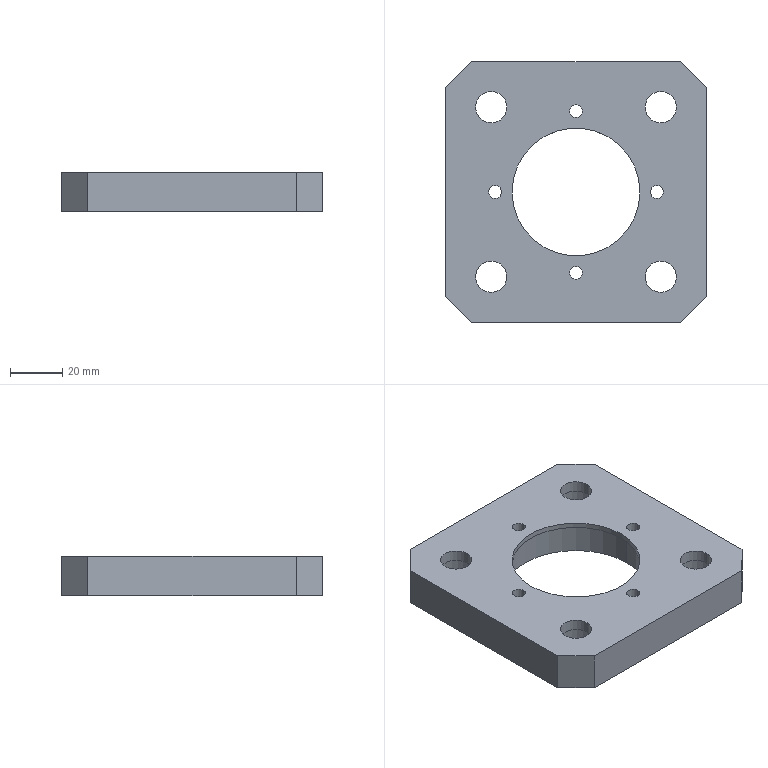Part | SolidWorks | features HoleWzd 2, ICE 2, Chamfer 1, Extrusion 1 | 1 solid | 43 faces | box 100 x 100 x 15 mm | volume 98385 mm3 | cylinder 28 | plane 15 | commonest cylinder face diameters 5 x8 12 x8 18 x8 49 x2 55 x2
STEP:
#1=CARTESIAN_POINT('',(24.5,0.,15.));
#2=VERTEX_POINT('',#1);
#3=CARTESIAN_POINT('',(-24.5,0.,15.));
#4=VERTEX_POINT('',#3);
#5=CARTESIAN_POINT('',(0.,0.,15.));
#6=DIRECTION('',(0.,0.,-1.));
#7=DIRECTION('',(-1.,0.,0.));
#8=AXIS2_PLACEMENT_3D('',#5,#6,#7);
#9=CIRCLE('',#8,24.5);
#10=EDGE_CURVE('',#2,#4,#9,.T.);
#11=ORIENTED_EDGE('',*,*,#10,.F.);
#12=CARTESIAN_POINT('',(24.5,0.,13.));
#13=VERTEX_POINT('',#12);
#14=CARTESIAN_POINT('',(24.5,0.,15.));
#15=DIRECTION('',(0.,0.,-1.));
#16=VECTOR('',#15,1000.);
#17=LINE('',#14,#16);
#18=EDGE_CURVE('',#2,#13,#17,.T.);
#19=ORIENTED_EDGE('',*,*,#18,.T.);
#20=CARTESIAN_POINT('',(-24.5,0.,13.));
#21=VERTEX_POINT('',#20);
#22=CARTESIAN_POINT('',(0.,0.,13.));
#23=DIRECTION('',(0.,0.,-1.));
#24=DIRECTION('',(-1.,0.,0.));
#25=AXIS2_PLACEMENT_3D('',#22,#23,#24);
#26=CIRCLE('',#25,24.5);
#27=EDGE_CURVE('',#13,#21,#26,.T.);
#28=ORIENTED_EDGE('',*,*,#27,.T.);
#29=CARTESIAN_POINT('',(-24.5,0.,15.));
#30=DIRECTION('',(0.,0.,-1.));
#31=VECTOR('',#30,1000.);
#32=LINE('',#29,#31);
#33=EDGE_CURVE('',#4,#21,#32,.T.);
#34=ORIENTED_EDGE('',*,*,#33,.F.);
#35=EDGE_LOOP('',(#11,#19,#28,#34));
#36=FACE_OUTER_BOUND('',#35,.T.);
#37=CARTESIAN_POINT('',(0.,0.,15.));
#38=DIRECTION('',(0.,0.,-1.));
#39=DIRECTION('',(-1.,0.,0.));
#40=AXIS2_PLACEMENT_3D('',#37,#38,#39);
#41=CYLINDRICAL_SURFACE('',#40,24.5);
#42=ADVANCED_FACE('',(#36),#41,.F.);
#43=CARTESIAN_POINT('',(2.5,31.,15.));
#44=VERTEX_POINT('',#43);
#45=CARTESIAN_POINT('',(-2.5,31.,15.));
#46=VERTEX_POINT('',#45);
#47=CARTESIAN_POINT('',(0.,31.,15.));
#48=DIRECTION('',(0.,0.,-1.));
#49=DIRECTION('',(-1.,0.,0.));
#50=AXIS2_PLACEMENT_3D('',#47,#48,#49);
#51=CIRCLE('',#50,2.5);
#52=EDGE_CURVE('',#44,#46,#51,.T.);
#53=ORIENTED_EDGE('',*,*,#52,.F.);
#54=CARTESIAN_POINT('',(2.5,31.,0.));
#55=VERTEX_POINT('',#54);
#56=CARTESIAN_POINT('',(2.5,31.,0.));
#57=DIRECTION('',(0.,0.,-1.));
#58=VECTOR('',#57,1000.);
#59=LINE('',#56,#58);
#60=EDGE_CURVE('',#44,#55,#59,.T.);
#61=ORIENTED_EDGE('',*,*,#60,.T.);
#62=CARTESIAN_POINT('',(-2.5,31.,0.));
#63=VERTEX_POINT('',#62);
#64=CARTESIAN_POINT('',(0.,31.,0.));
#65=DIRECTION('',(0.,0.,-1.));
#66=DIRECTION('',(-1.,0.,0.));
#67=AXIS2_PLACEMENT_3D('',#64,#65,#66);
#68=CIRCLE('',#67,2.5);
#69=EDGE_CURVE('',#55,#63,#68,.T.);
#70=ORIENTED_EDGE('',*,*,#69,.T.);
#71=CARTESIAN_POINT('',(-2.5,31.,0.));
#72=DIRECTION('',(0.,0.,-1.));
#73=VECTOR('',#72,1000.);
#74=LINE('',#71,#73);
#75=EDGE_CURVE('',#46,#63,#74,.T.);
#76=ORIENTED_EDGE('',*,*,#75,.F.);
#77=EDGE_LOOP('',(#53,#61,#70,#76));
#78=FACE_OUTER_BOUND('',#77,.T.);
#79=CARTESIAN_POINT('',(0.,31.,0.));
#80=DIRECTION('',(0.,0.,-1.));
#81=DIRECTION('',(-1.,0.,0.));
#82=AXIS2_PLACEMENT_3D('',#79,#80,#81);
#83=CYLINDRICAL_SURFACE('',#82,2.5);
#84=ADVANCED_FACE('',(#78),#83,.F.);
#85=CARTESIAN_POINT('',(-28.5,0.,15.));
#86=VERTEX_POINT('',#85);
#87=CARTESIAN_POINT('',(-33.5,0.,15.));
#88=VERTEX_POINT('',#87);
#89=CARTESIAN_POINT('',(-31.,0.,15.));
#90=DIRECTION('',(0.,0.,-1.));
#91=DIRECTION('',(-1.,0.,0.));
#92=AXIS2_PLACEMENT_3D('',#89,#90,#91);
#93=CIRCLE('',#92,2.5);
#94=EDGE_CURVE('',#86,#88,#93,.T.);
#95=ORIENTED_EDGE('',*,*,#94,.F.);
#96=CARTESIAN_POINT('',(-28.5,0.,0.));
#97=VERTEX_POINT('',#96);
#98=CARTESIAN_POINT('',(-28.5,0.,0.));
#99=DIRECTION('',(0.,0.,-1.));
#100=VECTOR('',#99,1000.);
#101=LINE('',#98,#100);
#102=EDGE_CURVE('',#86,#97,#101,.T.);
#103=ORIENTED_EDGE('',*,*,#102,.T.);
#104=CARTESIAN_POINT('',(-33.5,0.,0.));
#105=VERTEX_POINT('',#104);
#106=CARTESIAN_POINT('',(-31.,0.,0.));
#107=DIRECTION('',(0.,0.,-1.));
#108=DIRECTION('',(-1.,0.,0.));
#109=AXIS2_PLACEMENT_3D('',#106,#107,#108);
#110=CIRCLE('',#109,2.5);
#111=EDGE_CURVE('',#97,#105,#110,.T.);
#112=ORIENTED_EDGE('',*,*,#111,.T.);
#113=CARTESIAN_POINT('',(-33.5,0.,0.));
#114=DIRECTION('',(0.,0.,-1.));
#115=VECTOR('',#114,1000.);
#116=LINE('',#113,#115);
#117=EDGE_CURVE('',#88,#105,#116,.T.);
#118=ORIENTED_EDGE('',*,*,#117,.F.);
#119=EDGE_LOOP('',(#95,#103,#112,#118));
#120=FACE_OUTER_BOUND('',#119,.T.);
#121=CARTESIAN_POINT('',(-31.,0.,0.));
#122=DIRECTION('',(0.,0.,-1.));
#123=DIRECTION('',(-1.,0.,0.));
#124=AXIS2_PLACEMENT_3D('',#121,#122,#123);
#125=CYLINDRICAL_SURFACE('',#124,2.5);
#126=ADVANCED_FACE('',(#120),#125,.F.);
#127=CARTESIAN_POINT('',(2.5,-31.,15.));
#128=VERTEX_POINT('',#127);
#129=CARTESIAN_POINT('',(-2.5,-31.,15.));
#130=VERTEX_POINT('',#129);
#131=CARTESIAN_POINT('',(0.,-31.,15.));
#132=DIRECTION('',(0.,0.,-1.));
#133=DIRECTION('',(-1.,0.,0.));
#134=AXIS2_PLACEMENT_3D('',#131,#132,#133);
#135=CIRCLE('',#134,2.5);
#136=EDGE_CURVE('',#128,#130,#135,.T.);
#137=ORIENTED_EDGE('',*,*,#136,.F.);
#138=CARTESIAN_POINT('',(2.5,-31.,0.));
#139=VERTEX_POINT('',#138);
#140=CARTESIAN_POINT('',(2.5,-31.,0.));
#141=DIRECTION('',(0.,0.,-1.));
#142=VECTOR('',#141,1000.);
#143=LINE('',#140,#142);
#144=EDGE_CURVE('',#128,#139,#143,.T.);
#145=ORIENTED_EDGE('',*,*,#144,.T.);
#146=CARTESIAN_POINT('',(-2.5,-31.,0.));
#147=VERTEX_POINT('',#146);
#148=CARTESIAN_POINT('',(0.,-31.,0.));
#149=DIRECTION('',(0.,0.,-1.));
#150=DIRECTION('',(-1.,0.,0.));
#151=AXIS2_PLACEMENT_3D('',#148,#149,#150);
#152=CIRCLE('',#151,2.5);
#153=EDGE_CURVE('',#139,#147,#152,.T.);
#154=ORIENTED_EDGE('',*,*,#153,.T.);
#155=CARTESIAN_POINT('',(-2.5,-31.,0.));
#156=DIRECTION('',(0.,0.,-1.));
#157=VECTOR('',#156,1000.);
#158=LINE('',#155,#157);
#159=EDGE_CURVE('',#130,#147,#158,.T.);
#160=ORIENTED_EDGE('',*,*,#159,.F.);
#161=EDGE_LOOP('',(#137,#145,#154,#160));
#162=FACE_OUTER_BOUND('',#161,.T.);
#163=CARTESIAN_POINT('',(0.,-31.,0.));
#164=DIRECTION('',(0.,0.,-1.));
#165=DIRECTION('',(-1.,0.,0.));
#166=AXIS2_PLACEMENT_3D('',#163,#164,#165);
#167=CYLINDRICAL_SURFACE('',#166,2.5);
#168=ADVANCED_FACE('',(#162),#167,.F.);
#169=CARTESIAN_POINT('',(33.5,0.,15.));
#170=VERTEX_POINT('',#169);
#171=CARTESIAN_POINT('',(28.5,0.,15.));
#172=VERTEX_POINT('',#171);
#173=CARTESIAN_POINT('',(31.,0.,15.));
#174=DIRECTION('',(0.,0.,-1.));
#175=DIRECTION('',(-1.,0.,0.));
#176=AXIS2_PLACEMENT_3D('',#173,#174,#175);
#177=CIRCLE('',#176,2.5);
#178=EDGE_CURVE('',#170,#172,#177,.T.);
#179=ORIENTED_EDGE('',*,*,#178,.F.);
#180=CARTESIAN_POINT('',(33.5,0.,0.));
#181=VERTEX_POINT('',#180);
#182=CARTESIAN_POINT('',(33.5,0.,0.));
#183=DIRECTION('',(0.,0.,-1.));
#184=VECTOR('',#183,1000.);
#185=LINE('',#182,#184);
#186=EDGE_CURVE('',#170,#181,#185,.T.);
#187=ORIENTED_EDGE('',*,*,#186,.T.);
#188=CARTESIAN_POINT('',(28.5,0.,0.));
#189=VERTEX_POINT('',#188);
#190=CARTESIAN_POINT('',(31.,0.,0.));
#191=DIRECTION('',(0.,0.,-1.));
#192=DIRECTION('',(-1.,0.,0.));
#193=AXIS2_PLACEMENT_3D('',#190,#191,#192);
#194=CIRCLE('',#193,2.5);
#195=EDGE_CURVE('',#181,#189,#194,.T.);
#196=ORIENTED_EDGE('',*,*,#195,.T.);
#197=CARTESIAN_POINT('',(28.5,0.,0.));
#198=DIRECTION('',(0.,0.,-1.));
#199=VECTOR('',#198,1000.);
#200=LINE('',#197,#199);
#201=EDGE_CURVE('',#172,#189,#200,.T.);
#202=ORIENTED_EDGE('',*,*,#201,.F.);
#203=EDGE_LOOP('',(#179,#187,#196,#202));
#204=FACE_OUTER_BOUND('',#203,.T.);
#205=CARTESIAN_POINT('',(31.,0.,0.));
#206=DIRECTION('',(0.,0.,-1.));
#207=DIRECTION('',(-1.,0.,0.));
#208=AXIS2_PLACEMENT_3D('',#205,#206,#207);
#209=CYLINDRICAL_SURFACE('',#208,2.5);
#210=ADVANCED_FACE('',(#204),#209,.F.);
#211=CARTESIAN_POINT('',(27.5,0.,13.));
#212=VERTEX_POINT('',#211);
#213=CARTESIAN_POINT('',(-27.5,0.,13.));
#214=VERTEX_POINT('',#213);
#215=CARTESIAN_POINT('',(0.,0.,13.));
#216=DIRECTION('',(0.,0.,-1.));
#217=DIRECTION('',(-1.,0.,0.));
#218=AXIS2_PLACEMENT_3D('',#215,#216,#217);
#219=CIRCLE('',#218,27.5);
#220=EDGE_CURVE('',#212,#214,#219,.T.);
#221=ORIENTED_EDGE('',*,*,#220,.F.);
#222=CARTESIAN_POINT('',(27.5,0.,0.));
#223=VERTEX_POINT('',#222);
#224=CARTESIAN_POINT('',(27.5,0.,13.));
#225=DIRECTION('',(0.,0.,-1.));
#226=VECTOR('',#225,1000.);
#227=LINE('',#224,#226);
#228=EDGE_CURVE('',#212,#223,#227,.T.);
#229=ORIENTED_EDGE('',*,*,#228,.T.);
#230=CARTESIAN_POINT('',(-27.5,0.,0.));
#231=VERTEX_POINT('',#230);
#232=CARTESIAN_POINT('',(0.,0.,0.));
#233=DIRECTION('',(0.,0.,-1.));
#234=DIRECTION('',(-1.,0.,0.));
#235=AXIS2_PLACEMENT_3D('',#232,#233,#234);
#236=CIRCLE('',#235,27.5);
#237=EDGE_CURVE('',#223,#231,#236,.T.);
#238=ORIENTED_EDGE('',*,*,#237,.T.);
#239=CARTESIAN_POINT('',(-27.5,0.,13.));
#240=DIRECTION('',(0.,0.,-1.));
#241=VECTOR('',#240,1000.);
#242=LINE('',#239,#241);
#243=EDGE_CURVE('',#214,#231,#242,.T.);
#244=ORIENTED_EDGE('',*,*,#243,.F.);
#245=EDGE_LOOP('',(#221,#229,#238,#244));
#246=FACE_OUTER_BOUND('',#245,.T.);
#247=CARTESIAN_POINT('',(0.,0.,13.));
#248=DIRECTION('',(0.,0.,-1.));
#249=DIRECTION('',(-1.,0.,0.));
#250=AXIS2_PLACEMENT_3D('',#247,#248,#249);
#251=CYLINDRICAL_SURFACE('',#250,27.5);
#252=ADVANCED_FACE('',(#246),#251,.F.);
#253=CARTESIAN_POINT('',(41.5,32.5,10.6));
#254=VERTEX_POINT('',#253);
#255=CARTESIAN_POINT('',(23.5,32.5,10.6));
#256=VERTEX_POINT('',#255);
#257=CARTESIAN_POINT('',(32.5,32.5,10.6));
#258=DIRECTION('',(0.,0.,-1.));
#259=DIRECTION('',(-1.,0.,0.));
#260=AXIS2_PLACEMENT_3D('',#257,#258,#259);
#261=CIRCLE('',#260,9.);
#262=EDGE_CURVE('',#254,#256,#261,.T.);
#263=ORIENTED_EDGE('',*,*,#262,.F.);
#264=CARTESIAN_POINT('',(41.5,32.5,0.));
#265=VERTEX_POINT('',#264);
#266=CARTESIAN_POINT('',(41.5,32.5,0.));
#267=DIRECTION('',(0.,0.,-1.));
#268=VECTOR('',#267,1000.);
#269=LINE('',#266,#268);
#270=EDGE_CURVE('',#254,#265,#269,.T.);
#271=ORIENTED_EDGE('',*,*,#270,.T.);
#272=CARTESIAN_POINT('',(23.5,32.5,0.));
#273=VERTEX_POINT('',#272);
#274=CARTESIAN_POINT('',(32.5,32.5,0.));
#275=DIRECTION('',(0.,0.,-1.));
#276=DIRECTION('',(-1.,0.,0.));
#277=AXIS2_PLACEMENT_3D('',#274,#275,#276);
#278=CIRCLE('',#277,9.);
#279=EDGE_CURVE('',#265,#273,#278,.T.);
#280=ORIENTED_EDGE('',*,*,#279,.T.);
#281=CARTESIAN_POINT('',(23.5,32.5,0.));
#282=DIRECTION('',(0.,0.,-1.));
#283=VECTOR('',#282,1000.);
#284=LINE('',#281,#283);
#285=EDGE_CURVE('',#256,#273,#284,.T.);
#286=ORIENTED_EDGE('',*,*,#285,.F.);
#287=EDGE_LOOP('',(#263,#271,#280,#286));
#288=FACE_OUTER_BOUND('',#287,.T.);
#289=CARTESIAN_POINT('',(32.5,32.5,0.));
#290=DIRECTION('',(0.,0.,-1.));
#291=DIRECTION('',(-1.,0.,0.));
#292=AXIS2_PLACEMENT_3D('',#289,#290,#291);
#293=CYLINDRICAL_SURFACE('',#292,9.);
#294=ADVANCED_FACE('',(#288),#293,.F.);
#295=CARTESIAN_POINT('',(38.5,32.5,15.));
#296=VERTEX_POINT('',#295);
#297=CARTESIAN_POINT('',(26.5,32.5,15.));
#298=VERTEX_POINT('',#297);
#299=CARTESIAN_POINT('',(32.5,32.5,15.));
#300=DIRECTION('',(0.,0.,-1.));
#301=DIRECTION('',(-1.,0.,0.));
#302=AXIS2_PLACEMENT_3D('',#299,#300,#301);
#303=CIRCLE('',#302,6.);
#304=EDGE_CURVE('',#296,#298,#303,.T.);
#305=ORIENTED_EDGE('',*,*,#304,.F.);
#306=CARTESIAN_POINT('',(38.5,32.5,10.6));
#307=VERTEX_POINT('',#306);
#308=CARTESIAN_POINT('',(38.5,32.5,0.));
#309=DIRECTION('',(0.,0.,-1.));
#310=VECTOR('',#309,1000.);
#311=LINE('',#308,#310);
#312=EDGE_CURVE('',#296,#307,#311,.T.);
#313=ORIENTED_EDGE('',*,*,#312,.T.);
#314=CARTESIAN_POINT('',(26.5,32.5,10.6));
#315=VERTEX_POINT('',#314);
#316=CARTESIAN_POINT('',(32.5,32.5,10.6));
#317=DIRECTION('',(0.,0.,-1.));
#318=DIRECTION('',(-1.,0.,0.));
#319=AXIS2_PLACEMENT_3D('',#316,#317,#318);
#320=CIRCLE('',#319,6.);
#321=EDGE_CURVE('',#307,#315,#320,.T.);
#322=ORIENTED_EDGE('',*,*,#321,.T.);
#323=CARTESIAN_POINT('',(26.5,32.5,0.));
#324=DIRECTION('',(0.,0.,-1.));
#325=VECTOR('',#324,1000.);
#326=LINE('',#323,#325);
#327=EDGE_CURVE('',#298,#315,#326,.T.);
#328=ORIENTED_EDGE('',*,*,#327,.F.);
#329=EDGE_LOOP('',(#305,#313,#322,#328));
#330=FACE_OUTER_BOUND('',#329,.T.);
#331=CARTESIAN_POINT('',(32.5,32.5,0.));
#332=DIRECTION('',(0.,0.,-1.));
#333=DIRECTION('',(-1.,0.,0.));
#334=AXIS2_PLACEMENT_3D('',#331,#332,#333);
#335=CYLINDRICAL_SURFACE('',#334,6.);
#336=ADVANCED_FACE('',(#330),#335,.F.);
#337=CARTESIAN_POINT('',(-23.5,32.5,10.6));
#338=VERTEX_POINT('',#337);
#339=CARTESIAN_POINT('',(-41.5,32.5,10.6));
#340=VERTEX_POINT('',#339);
#341=CARTESIAN_POINT('',(-32.5,32.5,10.6));
#342=DIRECTION('',(0.,0.,-1.));
#343=DIRECTION('',(-1.,0.,0.));
#344=AXIS2_PLACEMENT_3D('',#341,#342,#343);
#345=CIRCLE('',#344,9.);
#346=EDGE_CURVE('',#338,#340,#345,.T.);
#347=ORIENTED_EDGE('',*,*,#346,.F.);
#348=CARTESIAN_POINT('',(-23.5,32.5,0.));
#349=VERTEX_POINT('',#348);
#350=CARTESIAN_POINT('',(-23.5,32.5,0.));
#351=DIRECTION('',(0.,0.,-1.));
#352=VECTOR('',#351,1000.);
#353=LINE('',#350,#352);
#354=EDGE_CURVE('',#338,#349,#353,.T.);
#355=ORIENTED_EDGE('',*,*,#354,.T.);
#356=CARTESIAN_POINT('',(-41.5,32.5,0.));
#357=VERTEX_POINT('',#356);
#358=CARTESIAN_POINT('',(-32.5,32.5,0.));
#359=DIRECTION('',(0.,0.,-1.));
#360=DIRECTION('',(-1.,0.,0.));
#361=AXIS2_PLACEMENT_3D('',#358,#359,#360);
#362=CIRCLE('',#361,9.);
#363=EDGE_CURVE('',#349,#357,#362,.T.);
#364=ORIENTED_EDGE('',*,*,#363,.T.);
#365=CARTESIAN_POINT('',(-41.5,32.5,0.));
#366=DIRECTION('',(0.,0.,-1.));
#367=VECTOR('',#366,1000.);
#368=LINE('',#365,#367);
#369=EDGE_CURVE('',#340,#357,#368,.T.);
#370=ORIENTED_EDGE('',*,*,#369,.F.);
#371=EDGE_LOOP('',(#347,#355,#364,#370));
#372=FACE_OUTER_BOUND('',#371,.T.);
#373=CARTESIAN_POINT('',(-32.5,32.5,0.));
#374=DIRECTION('',(0.,0.,-1.));
#375=DIRECTION('',(-1.,0.,0.));
#376=AXIS2_PLACEMENT_3D('',#373,#374,#375);
#377=CYLINDRICAL_SURFACE('',#376,9.);
#378=ADVANCED_FACE('',(#372),#377,.F.);
#379=CARTESIAN_POINT('',(-26.5,32.5,15.));
#380=VERTEX_POINT('',#379);
#381=CARTESIAN_POINT('',(-38.5,32.5,15.));
#382=VERTEX_POINT('',#381);
#383=CARTESIAN_POINT('',(-32.5,32.5,15.));
#384=DIRECTION('',(0.,0.,-1.));
#385=DIRECTION('',(-1.,0.,0.));
#386=AXIS2_PLACEMENT_3D('',#383,#384,#385);
#387=CIRCLE('',#386,6.);
#388=EDGE_CURVE('',#380,#382,#387,.T.);
#389=ORIENTED_EDGE('',*,*,#388,.F.);
#390=CARTESIAN_POINT('',(-26.5,32.5,10.6));
#391=VERTEX_POINT('',#390);
#392=CARTESIAN_POINT('',(-26.5,32.5,0.));
#393=DIRECTION('',(0.,0.,-1.));
#394=VECTOR('',#393,1000.);
#395=LINE('',#392,#394);
#396=EDGE_CURVE('',#380,#391,#395,.T.);
#397=ORIENTED_EDGE('',*,*,#396,.T.);
#398=CARTESIAN_POINT('',(-38.5,32.5,10.6));
#399=VERTEX_POINT('',#398);
#400=CARTESIAN_POINT('',(-32.5,32.5,10.6));
#401=DIRECTION('',(0.,0.,-1.));
#402=DIRECTION('',(-1.,0.,0.));
#403=AXIS2_PLACEMENT_3D('',#400,#401,#402);
#404=CIRCLE('',#403,6.);
#405=EDGE_CURVE('',#391,#399,#404,.T.);
#406=ORIENTED_EDGE('',*,*,#405,.T.);
#407=CARTESIAN_POINT('',(-38.5,32.5,0.));
#408=DIRECTION('',(0.,0.,-1.));
#409=VECTOR('',#408,1000.);
#410=LINE('',#407,#409);
#411=EDGE_CURVE('',#382,#399,#410,.T.);
#412=ORIENTED_EDGE('',*,*,#411,.F.);
#413=EDGE_LOOP('',(#389,#397,#406,#412));
#414=FACE_OUTER_BOUND('',#413,.T.);
#415=CARTESIAN_POINT('',(-32.5,32.5,0.));
#416=DIRECTION('',(0.,0.,-1.));
#417=DIRECTION('',(-1.,0.,0.));
#418=AXIS2_PLACEMENT_3D('',#415,#416,#417);
#419=CYLINDRICAL_SURFACE('',#418,6.);
#420=ADVANCED_FACE('',(#414),#419,.F.);
#421=CARTESIAN_POINT('',(-23.5,-32.5,10.6));
#422=VERTEX_POINT('',#421);
#423=CARTESIAN_POINT('',(-41.5,-32.5,10.6));
#424=VERTEX_POINT('',#423);
#425=CARTESIAN_POINT('',(-32.5,-32.5,10.6));
#426=DIRECTION('',(0.,0.,-1.));
#427=DIRECTION('',(-1.,0.,0.));
#428=AXIS2_PLACEMENT_3D('',#425,#426,#427);
#429=CIRCLE('',#428,9.);
#430=EDGE_CURVE('',#422,#424,#429,.T.);
#431=ORIENTED_EDGE('',*,*,#430,.F.);
#432=CARTESIAN_POINT('',(-23.5,-32.5,0.));
#433=VERTEX_POINT('',#432);
#434=CARTESIAN_POINT('',(-23.5,-32.5,0.));
#435=DIRECTION('',(0.,0.,-1.));
#436=VECTOR('',#435,1000.);
#437=LINE('',#434,#436);
#438=EDGE_CURVE('',#422,#433,#437,.T.);
#439=ORIENTED_EDGE('',*,*,#438,.T.);
#440=CARTESIAN_POINT('',(-41.5,-32.5,0.));
#441=VERTEX_POINT('',#440);
#442=CARTESIAN_POINT('',(-32.5,-32.5,0.));
#443=DIRECTION('',(0.,0.,-1.));
#444=DIRECTION('',(-1.,0.,0.));
#445=AXIS2_PLACEMENT_3D('',#442,#443,#444);
#446=CIRCLE('',#445,9.);
#447=EDGE_CURVE('',#433,#441,#446,.T.);
#448=ORIENTED_EDGE('',*,*,#447,.T.);
#449=CARTESIAN_POINT('',(-41.5,-32.5,0.));
#450=DIRECTION('',(0.,0.,-1.));
#451=VECTOR('',#450,1000.);
#452=LINE('',#449,#451);
#453=EDGE_CURVE('',#424,#441,#452,.T.);
#454=ORIENTED_EDGE('',*,*,#453,.F.);
#455=EDGE_LOOP('',(#431,#439,#448,#454));
#456=FACE_OUTER_BOUND('',#455,.T.);
#457=CARTESIAN_POINT('',(-32.5,-32.5,0.));
#458=DIRECTION('',(0.,0.,-1.));
#459=DIRECTION('',(-1.,0.,0.));
#460=AXIS2_PLACEMENT_3D('',#457,#458,#459);
#461=CYLINDRICAL_SURFACE('',#460,9.);
#462=ADVANCED_FACE('',(#456),#461,.F.);
#463=CARTESIAN_POINT('',(-26.5,-32.5,15.));
#464=VERTEX_POINT('',#463);
#465=CARTESIAN_POINT('',(-38.5,-32.5,15.));
#466=VERTEX_POINT('',#465);
#467=CARTESIAN_POINT('',(-32.5,-32.5,15.));
#468=DIRECTION('',(0.,0.,-1.));
#469=DIRECTION('',(-1.,0.,0.));
#470=AXIS2_PLACEMENT_3D('',#467,#468,#469);
#471=CIRCLE('',#470,6.);
#472=EDGE_CURVE('',#464,#466,#471,.T.);
#473=ORIENTED_EDGE('',*,*,#472,.F.);
#474=CARTESIAN_POINT('',(-26.5,-32.5,10.6));
#475=VERTEX_POINT('',#474);
#476=CARTESIAN_POINT('',(-26.5,-32.5,0.));
#477=DIRECTION('',(0.,0.,-1.));
#478=VECTOR('',#477,1000.);
#479=LINE('',#476,#478);
#480=EDGE_CURVE('',#464,#475,#479,.T.);
#481=ORIENTED_EDGE('',*,*,#480,.T.);
#482=CARTESIAN_POINT('',(-38.5,-32.5,10.6));
#483=VERTEX_POINT('',#482);
#484=CARTESIAN_POINT('',(-32.5,-32.5,10.6));
#485=DIRECTION('',(0.,0.,-1.));
#486=DIRECTION('',(-1.,0.,0.));
#487=AXIS2_PLACEMENT_3D('',#484,#485,#486);
#488=CIRCLE('',#487,6.);
#489=EDGE_CURVE('',#475,#483,#488,.T.);
#490=ORIENTED_EDGE('',*,*,#489,.T.);
#491=CARTESIAN_POINT('',(-38.5,-32.5,0.));
#492=DIRECTION('',(0.,0.,-1.));
#493=VECTOR('',#492,1000.);
#494=LINE('',#491,#493);
#495=EDGE_CURVE('',#466,#483,#494,.T.);
#496=ORIENTED_EDGE('',*,*,#495,.F.);
#497=EDGE_LOOP('',(#473,#481,#490,#496));
#498=FACE_OUTER_BOUND('',#497,.T.);
#499=CARTESIAN_POINT('',(-32.5,-32.5,0.));
#500=DIRECTION('',(0.,0.,-1.));
#501=DIRECTION('',(-1.,0.,0.));
#502=AXIS2_PLACEMENT_3D('',#499,#500,#501);
#503=CYLINDRICAL_SURFACE('',#502,6.);
#504=ADVANCED_FACE('',(#498),#503,.F.);
#505=CARTESIAN_POINT('',(41.5,-32.5,10.6));
#506=VERTEX_POINT('',#505);
#507=CARTESIAN_POINT('',(23.5,-32.5,10.6));
#508=VERTEX_POINT('',#507);
#509=CARTESIAN_POINT('',(32.5,-32.5,10.6));
#510=DIRECTION('',(0.,0.,-1.));
#511=DIRECTION('',(-1.,0.,0.));
#512=AXIS2_PLACEMENT_3D('',#509,#510,#511);
#513=CIRCLE('',#512,9.);
#514=EDGE_CURVE('',#506,#508,#513,.T.);
#515=ORIENTED_EDGE('',*,*,#514,.F.);
#516=CARTESIAN_POINT('',(41.5,-32.5,0.));
#517=VERTEX_POINT('',#516);
#518=CARTESIAN_POINT('',(41.5,-32.5,0.));
#519=DIRECTION('',(0.,0.,-1.));
#520=VECTOR('',#519,1000.);
#521=LINE('',#518,#520);
#522=EDGE_CURVE('',#506,#517,#521,.T.);
#523=ORIENTED_EDGE('',*,*,#522,.T.);
#524=CARTESIAN_POINT('',(23.5,-32.5,0.));
#525=VERTEX_POINT('',#524);
#526=CARTESIAN_POINT('',(32.5,-32.5,0.));
#527=DIRECTION('',(0.,0.,-1.));
#528=DIRECTION('',(-1.,0.,0.));
#529=AXIS2_PLACEMENT_3D('',#526,#527,#528);
#530=CIRCLE('',#529,9.);
#531=EDGE_CURVE('',#517,#525,#530,.T.);
#532=ORIENTED_EDGE('',*,*,#531,.T.);
#533=CARTESIAN_POINT('',(23.5,-32.5,0.));
#534=DIRECTION('',(0.,0.,-1.));
#535=VECTOR('',#534,1000.);
#536=LINE('',#533,#535);
#537=EDGE_CURVE('',#508,#525,#536,.T.);
#538=ORIENTED_EDGE('',*,*,#537,.F.);
#539=EDGE_LOOP('',(#515,#523,#532,#538));
#540=FACE_OUTER_BOUND('',#539,.T.);
#541=CARTESIAN_POINT('',(32.5,-32.5,0.));
#542=DIRECTION('',(0.,0.,-1.));
#543=DIRECTION('',(-1.,0.,0.));
#544=AXIS2_PLACEMENT_3D('',#541,#542,#543);
#545=CYLINDRICAL_SURFACE('',#544,9.);
#546=ADVANCED_FACE('',(#540),#545,.F.);
#547=CARTESIAN_POINT('',(38.5,-32.5,15.));
#548=VERTEX_POINT('',#547);
#549=CARTESIAN_POINT('',(26.5,-32.5,15.));
#550=VERTEX_POINT('',#549);
#551=CARTESIAN_POINT('',(32.5,-32.5,15.));
#552=DIRECTION('',(0.,0.,-1.));
#553=DIRECTION('',(-1.,0.,0.));
#554=AXIS2_PLACEMENT_3D('',#551,#552,#553);
#555=CIRCLE('',#554,6.);
#556=EDGE_CURVE('',#548,#550,#555,.T.);
#557=ORIENTED_EDGE('',*,*,#556,.F.);
#558=CARTESIAN_POINT('',(38.5,-32.5,10.6));
#559=VERTEX_POINT('',#558);
#560=CARTESIAN_POINT('',(38.5,-32.5,0.));
#561=DIRECTION('',(0.,0.,-1.));
#562=VECTOR('',#561,1000.);
#563=LINE('',#560,#562);
#564=EDGE_CURVE('',#548,#559,#563,.T.);
#565=ORIENTED_EDGE('',*,*,#564,.T.);
#566=CARTESIAN_POINT('',(26.5,-32.5,10.6));
#567=VERTEX_POINT('',#566);
#568=CARTESIAN_POINT('',(32.5,-32.5,10.6));
#569=DIRECTION('',(0.,0.,-1.));
#570=DIRECTION('',(-1.,0.,0.));
#571=AXIS2_PLACEMENT_3D('',#568,#569,#570);
#572=CIRCLE('',#571,6.);
#573=EDGE_CURVE('',#559,#567,#572,.T.);
#574=ORIENTED_EDGE('',*,*,#573,.T.);
#575=CARTESIAN_POINT('',(26.5,-32.5,0.));
#576=DIRECTION('',(0.,0.,-1.));
#577=VECTOR('',#576,1000.);
#578=LINE('',#575,#577);
#579=EDGE_CURVE('',#550,#567,#578,.T.);
#580=ORIENTED_EDGE('',*,*,#579,.F.);
#581=EDGE_LOOP('',(#557,#565,#574,#580));
#582=FACE_OUTER_BOUND('',#581,.T.);
#583=CARTESIAN_POINT('',(32.5,-32.5,0.));
#584=DIRECTION('',(0.,0.,-1.));
#585=DIRECTION('',(-1.,0.,0.));
#586=AXIS2_PLACEMENT_3D('',#583,#584,#585);
#587=CYLINDRICAL_SURFACE('',#586,6.);
#588=ADVANCED_FACE('',(#582),#587,.F.);
#589=CARTESIAN_POINT('',(50.,-40.,15.));
#590=VERTEX_POINT('',#589);
#591=CARTESIAN_POINT('',(50.,40.,15.));
#592=VERTEX_POINT('',#591);
#593=CARTESIAN_POINT('',(50.,-50.,15.));
#594=DIRECTION('',(0.,1.,0.));
#595=VECTOR('',#594,1000.);
#596=LINE('',#593,#595);
#597=EDGE_CURVE('',#590,#592,#596,.T.);
#598=ORIENTED_EDGE('',*,*,#597,.F.);
#599=CARTESIAN_POINT('',(50.,-40.,0.));
#600=VERTEX_POINT('',#599);
#601=CARTESIAN_POINT('',(50.,-40.,15.));
#602=DIRECTION('',(0.,0.,-1.));
#603=VECTOR('',#602,1000.);
#604=LINE('',#601,#603);
#605=EDGE_CURVE('',#590,#600,#604,.T.);
#606=ORIENTED_EDGE('',*,*,#605,.T.);
#607=CARTESIAN_POINT('',(50.,40.,0.));
#608=VERTEX_POINT('',#607);
#609=CARTESIAN_POINT('',(50.,-50.,0.));
#610=DIRECTION('',(0.,1.,0.));
#611=VECTOR('',#610,1000.);
#612=LINE('',#609,#611);
#613=EDGE_CURVE('',#600,#608,#612,.T.);
#614=ORIENTED_EDGE('',*,*,#613,.T.);
#615=CARTESIAN_POINT('',(50.,40.,15.));
#616=DIRECTION('',(0.,0.,1.));
#617=VECTOR('',#616,1000.);
#618=LINE('',#615,#617);
#619=EDGE_CURVE('',#608,#592,#618,.T.);
#620=ORIENTED_EDGE('',*,*,#619,.T.);
#621=EDGE_LOOP('',(#598,#606,#614,#620));
#622=FACE_OUTER_BOUND('',#621,.T.);
#623=CARTESIAN_POINT('',(50.,-50.,15.));
#624=DIRECTION('',(-1.,0.,0.));
#625=DIRECTION('',(0.,0.,1.));
#626=AXIS2_PLACEMENT_3D('',#623,#624,#625);
#627=PLANE('',#626);
#628=ADVANCED_FACE('',(#622),#627,.F.);
#629=CARTESIAN_POINT('',(40.,50.,0.));
#630=VERTEX_POINT('',#629);
#631=CARTESIAN_POINT('',(-40.,50.,0.));
#632=VERTEX_POINT('',#631);
#633=CARTESIAN_POINT('',(-50.,50.,0.));
#634=DIRECTION('',(-1.,0.,0.));
#635=VECTOR('',#634,1000.);
#636=LINE('',#633,#635);
#637=EDGE_CURVE('',#630,#632,#636,.T.);
#638=ORIENTED_EDGE('',*,*,#637,.T.);
#639=CARTESIAN_POINT('',(-40.,50.,15.));
#640=VERTEX_POINT('',#639);
#641=CARTESIAN_POINT('',(-40.,50.,15.));
#642=DIRECTION('',(0.,0.,1.));
#643=VECTOR('',#642,1000.);
#644=LINE('',#641,#643);
#645=EDGE_CURVE('',#632,#640,#644,.T.);
#646=ORIENTED_EDGE('',*,*,#645,.T.);
#647=CARTESIAN_POINT('',(40.,50.,15.));
#648=VERTEX_POINT('',#647);
#649=CARTESIAN_POINT('',(-50.,50.,15.));
#650=DIRECTION('',(-1.,0.,0.));
#651=VECTOR('',#650,1000.);
#652=LINE('',#649,#651);
#653=EDGE_CURVE('',#648,#640,#652,.T.);
#654=ORIENTED_EDGE('',*,*,#653,.F.);
#655=CARTESIAN_POINT('',(40.,50.,15.));
#656=DIRECTION('',(0.,0.,-1.));
#657=VECTOR('',#656,1000.);
#658=LINE('',#655,#657);
#659=EDGE_CURVE('',#648,#630,#658,.T.);
#660=ORIENTED_EDGE('',*,*,#659,.T.);
#661=EDGE_LOOP('',(#638,#646,#654,#660));
#662=FACE_OUTER_BOUND('',#661,.T.);
#663=CARTESIAN_POINT('',(-50.,50.,15.));
#664=DIRECTION('',(0.,-1.,0.));
#665=DIRECTION('',(0.,0.,-1.));
#666=AXIS2_PLACEMENT_3D('',#663,#664,#665);
#667=PLANE('',#666);
#668=ADVANCED_FACE('',(#662),#667,.F.);
#669=CARTESIAN_POINT('',(-50.,40.,0.));
#670=VERTEX_POINT('',#669);
#671=CARTESIAN_POINT('',(-50.,-40.,0.));
#672=VERTEX_POINT('',#671);
#673=CARTESIAN_POINT('',(-50.,-50.,0.));
#674=DIRECTION('',(0.,-1.,0.));
#675=VECTOR('',#674,1000.);
#676=LINE('',#673,#675);
#677=EDGE_CURVE('',#670,#672,#676,.T.);
#678=ORIENTED_EDGE('',*,*,#677,.T.);
#679=CARTESIAN_POINT('',(-50.,-40.,15.));
#680=VERTEX_POINT('',#679);
#681=CARTESIAN_POINT('',(-50.,-40.,15.));
#682=DIRECTION('',(0.,0.,1.));
#683=VECTOR('',#682,1000.);
#684=LINE('',#681,#683);
#685=EDGE_CURVE('',#672,#680,#684,.T.);
#686=ORIENTED_EDGE('',*,*,#685,.T.);
#687=CARTESIAN_POINT('',(-50.,40.,15.));
#688=VERTEX_POINT('',#687);
#689=CARTESIAN_POINT('',(-50.,-50.,15.));
#690=DIRECTION('',(0.,-1.,0.));
#691=VECTOR('',#690,1000.);
#692=LINE('',#689,#691);
#693=EDGE_CURVE('',#688,#680,#692,.T.);
#694=ORIENTED_EDGE('',*,*,#693,.F.);
#695=CARTESIAN_POINT('',(-50.,40.,15.));
#696=DIRECTION('',(0.,0.,-1.));
#697=VECTOR('',#696,1000.);
#698=LINE('',#695,#697);
#699=EDGE_CURVE('',#688,#670,#698,.T.);
#700=ORIENTED_EDGE('',*,*,#699,.T.);
#701=EDGE_LOOP('',(#678,#686,#694,#700));
#702=FACE_OUTER_BOUND('',#701,.T.);
#703=CARTESIAN_POINT('',(-50.,-50.,15.));
#704=DIRECTION('',(1.,0.,0.));
#705=DIRECTION('',(0.,0.,-1.));
#706=AXIS2_PLACEMENT_3D('',#703,#704,#705);
#707=PLANE('',#706);
#708=ADVANCED_FACE('',(#702),#707,.F.);
#709=CARTESIAN_POINT('',(-40.,-50.,0.));
#710=VERTEX_POINT('',#709);
#711=CARTESIAN_POINT('',(40.,-50.,0.));
#712=VERTEX_POINT('',#711);
#713=CARTESIAN_POINT('',(-50.,-50.,0.));
#714=DIRECTION('',(1.,0.,0.));
#715=VECTOR('',#714,1000.);
#716=LINE('',#713,#715);
#717=EDGE_CURVE('',#710,#712,#716,.T.);
#718=ORIENTED_EDGE('',*,*,#717,.T.);
#719=CARTESIAN_POINT('',(40.,-50.,15.));
#720=VERTEX_POINT('',#719);
#721=CARTESIAN_POINT('',(40.,-50.,15.));
#722=DIRECTION('',(0.,0.,1.));
#723=VECTOR('',#722,1000.);
#724=LINE('',#721,#723);
#725=EDGE_CURVE('',#712,#720,#724,.T.);
#726=ORIENTED_EDGE('',*,*,#725,.T.);
#727=CARTESIAN_POINT('',(-40.,-50.,15.));
#728=VERTEX_POINT('',#727);
#729=CARTESIAN_POINT('',(-50.,-50.,15.));
#730=DIRECTION('',(1.,0.,0.));
#731=VECTOR('',#730,1000.);
#732=LINE('',#729,#731);
#733=EDGE_CURVE('',#728,#720,#732,.T.);
#734=ORIENTED_EDGE('',*,*,#733,.F.);
#735=CARTESIAN_POINT('',(-40.,-50.,15.));
#736=DIRECTION('',(0.,0.,-1.));
#737=VECTOR('',#736,1000.);
#738=LINE('',#735,#737);
#739=EDGE_CURVE('',#728,#710,#738,.T.);
#740=ORIENTED_EDGE('',*,*,#739,.T.);
#741=EDGE_LOOP('',(#718,#726,#734,#740));
#742=FACE_OUTER_BOUND('',#741,.T.);
#743=CARTESIAN_POINT('',(-50.,-50.,15.));
#744=DIRECTION('',(0.,1.,0.));
#745=DIRECTION('',(0.,0.,1.));
#746=AXIS2_PLACEMENT_3D('',#743,#744,#745);
#747=PLANE('',#746);
#748=ADVANCED_FACE('',(#742),#747,.F.);
#749=CARTESIAN_POINT('',(0.,0.,15.));
#750=DIRECTION('',(0.,0.,-1.));
#751=DIRECTION('',(-1.,0.,0.));
#752=AXIS2_PLACEMENT_3D('',#749,#750,#751);
#753=CIRCLE('',#752,24.5);
#754=EDGE_CURVE('',#4,#2,#753,.T.);
#755=ORIENTED_EDGE('',*,*,#754,.T.);
#756=ORIENTED_EDGE('',*,*,#10,.T.);
#757=EDGE_LOOP('',(#755,#756));
#758=FACE_BOUND('',#757,.T.);
#759=CARTESIAN_POINT('',(0.,31.,15.));
#760=DIRECTION('',(0.,0.,-1.));
#761=DIRECTION('',(-1.,0.,0.));
#762=AXIS2_PLACEMENT_3D('',#759,#760,#761);
#763=CIRCLE('',#762,2.5);
#764=EDGE_CURVE('',#46,#44,#763,.T.);
#765=ORIENTED_EDGE('',*,*,#764,.T.);
#766=ORIENTED_EDGE('',*,*,#52,.T.);
#767=EDGE_LOOP('',(#765,#766));
#768=FACE_BOUND('',#767,.T.);
#769=CARTESIAN_POINT('',(-31.,0.,15.));
#770=DIRECTION('',(0.,0.,-1.));
#771=DIRECTION('',(-1.,0.,0.));
#772=AXIS2_PLACEMENT_3D('',#769,#770,#771);
#773=CIRCLE('',#772,2.5);
#774=EDGE_CURVE('',#88,#86,#773,.T.);
#775=ORIENTED_EDGE('',*,*,#774,.T.);
#776=ORIENTED_EDGE('',*,*,#94,.T.);
#777=EDGE_LOOP('',(#775,#776));
#778=FACE_BOUND('',#777,.T.);
#779=CARTESIAN_POINT('',(0.,-31.,15.));
#780=DIRECTION('',(0.,0.,-1.));
#781=DIRECTION('',(-1.,0.,0.));
#782=AXIS2_PLACEMENT_3D('',#779,#780,#781);
#783=CIRCLE('',#782,2.5);
#784=EDGE_CURVE('',#130,#128,#783,.T.);
#785=ORIENTED_EDGE('',*,*,#784,.T.);
#786=ORIENTED_EDGE('',*,*,#136,.T.);
#787=EDGE_LOOP('',(#785,#786));
#788=FACE_BOUND('',#787,.T.);
#789=CARTESIAN_POINT('',(31.,0.,15.));
#790=DIRECTION('',(0.,0.,-1.));
#791=DIRECTION('',(-1.,0.,0.));
#792=AXIS2_PLACEMENT_3D('',#789,#790,#791);
#793=CIRCLE('',#792,2.5);
#794=EDGE_CURVE('',#172,#170,#793,.T.);
#795=ORIENTED_EDGE('',*,*,#794,.T.);
#796=ORIENTED_EDGE('',*,*,#178,.T.);
#797=EDGE_LOOP('',(#795,#796));
#798=FACE_BOUND('',#797,.T.);
#799=CARTESIAN_POINT('',(32.5,32.5,15.));
#800=DIRECTION('',(0.,0.,-1.));
#801=DIRECTION('',(-1.,0.,0.));
#802=AXIS2_PLACEMENT_3D('',#799,#800,#801);
#803=CIRCLE('',#802,6.);
#804=EDGE_CURVE('',#298,#296,#803,.T.);
#805=ORIENTED_EDGE('',*,*,#804,.T.);
#806=ORIENTED_EDGE('',*,*,#304,.T.);
#807=EDGE_LOOP('',(#805,#806));
#808=FACE_BOUND('',#807,.T.);
#809=CARTESIAN_POINT('',(-32.5,32.5,15.));
#810=DIRECTION('',(0.,0.,-1.));
#811=DIRECTION('',(-1.,0.,0.));
#812=AXIS2_PLACEMENT_3D('',#809,#810,#811);
#813=CIRCLE('',#812,6.);
#814=EDGE_CURVE('',#382,#380,#813,.T.);
#815=ORIENTED_EDGE('',*,*,#814,.T.);
#816=ORIENTED_EDGE('',*,*,#388,.T.);
#817=EDGE_LOOP('',(#815,#816));
#818=FACE_BOUND('',#817,.T.);
#819=CARTESIAN_POINT('',(-32.5,-32.5,15.));
#820=DIRECTION('',(0.,0.,-1.));
#821=DIRECTION('',(-1.,0.,0.));
#822=AXIS2_PLACEMENT_3D('',#819,#820,#821);
#823=CIRCLE('',#822,6.);
#824=EDGE_CURVE('',#466,#464,#823,.T.);
#825=ORIENTED_EDGE('',*,*,#824,.T.);
#826=ORIENTED_EDGE('',*,*,#472,.T.);
#827=EDGE_LOOP('',(#825,#826));
#828=FACE_BOUND('',#827,.T.);
#829=CARTESIAN_POINT('',(32.5,-32.5,15.));
#830=DIRECTION('',(0.,0.,-1.));
#831=DIRECTION('',(-1.,0.,0.));
#832=AXIS2_PLACEMENT_3D('',#829,#830,#831);
#833=CIRCLE('',#832,6.);
#834=EDGE_CURVE('',#550,#548,#833,.T.);
#835=ORIENTED_EDGE('',*,*,#834,.T.);
#836=ORIENTED_EDGE('',*,*,#556,.T.);
#837=EDGE_LOOP('',(#835,#836));
#838=FACE_BOUND('',#837,.T.);
#839=ORIENTED_EDGE('',*,*,#733,.T.);
#840=CARTESIAN_POINT('',(50.,-40.,15.));
#841=DIRECTION('',(0.7071,0.7071,0.));
#842=VECTOR('',#841,1000.);
#843=LINE('',#840,#842);
#844=EDGE_CURVE('',#720,#590,#843,.T.);
#845=ORIENTED_EDGE('',*,*,#844,.T.);
#846=ORIENTED_EDGE('',*,*,#597,.T.);
#847=CARTESIAN_POINT('',(40.,50.,15.));
#848=DIRECTION('',(-0.7071,0.7071,0.));
#849=VECTOR('',#848,1000.);
#850=LINE('',#847,#849);
#851=EDGE_CURVE('',#592,#648,#850,.T.);
#852=ORIENTED_EDGE('',*,*,#851,.T.);
#853=ORIENTED_EDGE('',*,*,#653,.T.);
#854=CARTESIAN_POINT('',(-50.,40.,15.));
#855=DIRECTION('',(-0.7071,-0.7071,0.));
#856=VECTOR('',#855,1000.);
#857=LINE('',#854,#856);
#858=EDGE_CURVE('',#640,#688,#857,.T.);
#859=ORIENTED_EDGE('',*,*,#858,.T.);
#860=ORIENTED_EDGE('',*,*,#693,.T.);
#861=CARTESIAN_POINT('',(-40.,-50.,15.));
#862=DIRECTION('',(0.7071,-0.7071,0.));
#863=VECTOR('',#862,1000.);
#864=LINE('',#861,#863);
#865=EDGE_CURVE('',#680,#728,#864,.T.);
#866=ORIENTED_EDGE('',*,*,#865,.T.);
#867=EDGE_LOOP('',(#839,#845,#846,#852,#853,#859,#860,#866));
#868=FACE_OUTER_BOUND('',#867,.T.);
#869=CARTESIAN_POINT('',(0.,0.,15.));
#870=DIRECTION('',(0.,0.,-1.));
#871=DIRECTION('',(-1.,0.,0.));
#872=AXIS2_PLACEMENT_3D('',#869,#870,#871);
#873=PLANE('',#872);
#874=ADVANCED_FACE('',(#758,#768,#778,#788,#798,#808,#818,#828,#838,#868),#873,.F.);
#875=CARTESIAN_POINT('',(0.,31.,0.));
#876=DIRECTION('',(0.,0.,-1.));
#877=DIRECTION('',(-1.,0.,0.));
#878=AXIS2_PLACEMENT_3D('',#875,#876,#877);
#879=CIRCLE('',#878,2.5);
#880=EDGE_CURVE('',#63,#55,#879,.T.);
#881=ORIENTED_EDGE('',*,*,#880,.F.);
#882=ORIENTED_EDGE('',*,*,#69,.F.);
#883=EDGE_LOOP('',(#881,#882));
#884=FACE_BOUND('',#883,.T.);
#885=CARTESIAN_POINT('',(-31.,0.,0.));
#886=DIRECTION('',(0.,0.,-1.));
#887=DIRECTION('',(-1.,0.,0.));
#888=AXIS2_PLACEMENT_3D('',#885,#886,#887);
#889=CIRCLE('',#888,2.5);
#890=EDGE_CURVE('',#105,#97,#889,.T.);
#891=ORIENTED_EDGE('',*,*,#890,.F.);
#892=ORIENTED_EDGE('',*,*,#111,.F.);
#893=EDGE_LOOP('',(#891,#892));
#894=FACE_BOUND('',#893,.T.);
#895=CARTESIAN_POINT('',(0.,-31.,0.));
#896=DIRECTION('',(0.,0.,-1.));
#897=DIRECTION('',(-1.,0.,0.));
#898=AXIS2_PLACEMENT_3D('',#895,#896,#897);
#899=CIRCLE('',#898,2.5);
#900=EDGE_CURVE('',#147,#139,#899,.T.);
#901=ORIENTED_EDGE('',*,*,#900,.F.);
#902=ORIENTED_EDGE('',*,*,#153,.F.);
#903=EDGE_LOOP('',(#901,#902));
#904=FACE_BOUND('',#903,.T.);
#905=CARTESIAN_POINT('',(31.,0.,0.));
#906=DIRECTION('',(0.,0.,-1.));
#907=DIRECTION('',(-1.,0.,0.));
#908=AXIS2_PLACEMENT_3D('',#905,#906,#907);
#909=CIRCLE('',#908,2.5);
#910=EDGE_CURVE('',#189,#181,#909,.T.);
#911=ORIENTED_EDGE('',*,*,#910,.F.);
#912=ORIENTED_EDGE('',*,*,#195,.F.);
#913=EDGE_LOOP('',(#911,#912));
#914=FACE_BOUND('',#913,.T.);
#915=CARTESIAN_POINT('',(0.,0.,0.));
#916=DIRECTION('',(0.,0.,-1.));
#917=DIRECTION('',(-1.,0.,0.));
#918=AXIS2_PLACEMENT_3D('',#915,#916,#917);
#919=CIRCLE('',#918,27.5);
#920=EDGE_CURVE('',#231,#223,#919,.T.);
#921=ORIENTED_EDGE('',*,*,#920,.F.);
#922=ORIENTED_EDGE('',*,*,#237,.F.);
#923=EDGE_LOOP('',(#921,#922));
#924=FACE_BOUND('',#923,.T.);
#925=CARTESIAN_POINT('',(32.5,32.5,0.));
#926=DIRECTION('',(0.,0.,-1.));
#927=DIRECTION('',(-1.,0.,0.));
#928=AXIS2_PLACEMENT_3D('',#925,#926,#927);
#929=CIRCLE('',#928,9.);
#930=EDGE_CURVE('',#273,#265,#929,.T.);
#931=ORIENTED_EDGE('',*,*,#930,.F.);
#932=ORIENTED_EDGE('',*,*,#279,.F.);
#933=EDGE_LOOP('',(#931,#932));
#934=FACE_BOUND('',#933,.T.);
#935=CARTESIAN_POINT('',(-32.5,32.5,0.));
#936=DIRECTION('',(0.,0.,-1.));
#937=DIRECTION('',(-1.,0.,0.));
#938=AXIS2_PLACEMENT_3D('',#935,#936,#937);
#939=CIRCLE('',#938,9.);
#940=EDGE_CURVE('',#357,#349,#939,.T.);
#941=ORIENTED_EDGE('',*,*,#940,.F.);
#942=ORIENTED_EDGE('',*,*,#363,.F.);
#943=EDGE_LOOP('',(#941,#942));
#944=FACE_BOUND('',#943,.T.);
#945=CARTESIAN_POINT('',(-32.5,-32.5,0.));
#946=DIRECTION('',(0.,0.,-1.));
#947=DIRECTION('',(-1.,0.,0.));
#948=AXIS2_PLACEMENT_3D('',#945,#946,#947);
#949=CIRCLE('',#948,9.);
#950=EDGE_CURVE('',#441,#433,#949,.T.);
#951=ORIENTED_EDGE('',*,*,#950,.F.);
#952=ORIENTED_EDGE('',*,*,#447,.F.);
#953=EDGE_LOOP('',(#951,#952));
#954=FACE_BOUND('',#953,.T.);
#955=CARTESIAN_POINT('',(32.5,-32.5,0.));
#956=DIRECTION('',(0.,0.,-1.));
#957=DIRECTION('',(-1.,0.,0.));
#958=AXIS2_PLACEMENT_3D('',#955,#956,#957);
#959=CIRCLE('',#958,9.);
#960=EDGE_CURVE('',#525,#517,#959,.T.);
#961=ORIENTED_EDGE('',*,*,#960,.F.);
#962=ORIENTED_EDGE('',*,*,#531,.F.);
#963=EDGE_LOOP('',(#961,#962));
#964=FACE_BOUND('',#963,.T.);
#965=ORIENTED_EDGE('',*,*,#613,.F.);
#966=CARTESIAN_POINT('',(45.,-45.,0.));
#967=DIRECTION('',(-0.7071,-0.7071,0.));
#968=VECTOR('',#967,1000.);
#969=LINE('',#966,#968);
#970=EDGE_CURVE('',#600,#712,#969,.T.);
#971=ORIENTED_EDGE('',*,*,#970,.T.);
#972=ORIENTED_EDGE('',*,*,#717,.F.);
#973=CARTESIAN_POINT('',(-45.,-45.,0.));
#974=DIRECTION('',(-0.7071,0.7071,0.));
#975=VECTOR('',#974,1000.);
#976=LINE('',#973,#975);
#977=EDGE_CURVE('',#710,#672,#976,.T.);
#978=ORIENTED_EDGE('',*,*,#977,.T.);
#979=ORIENTED_EDGE('',*,*,#677,.F.);
#980=CARTESIAN_POINT('',(-45.,45.,0.));
#981=DIRECTION('',(0.7071,0.7071,0.));
#982=VECTOR('',#981,1000.);
#983=LINE('',#980,#982);
#984=EDGE_CURVE('',#670,#632,#983,.T.);
#985=ORIENTED_EDGE('',*,*,#984,.T.);
#986=ORIENTED_EDGE('',*,*,#637,.F.);
#987=CARTESIAN_POINT('',(45.,45.,0.));
#988=DIRECTION('',(0.7071,-0.7071,0.));
#989=VECTOR('',#988,1000.);
#990=LINE('',#987,#989);
#991=EDGE_CURVE('',#630,#608,#990,.T.);
#992=ORIENTED_EDGE('',*,*,#991,.T.);
#993=EDGE_LOOP('',(#965,#971,#972,#978,#979,#985,#986,#992));
#994=FACE_OUTER_BOUND('',#993,.T.);
#995=CARTESIAN_POINT('',(0.,0.,0.));
#996=DIRECTION('',(0.,0.,-1.));
#997=DIRECTION('',(-1.,0.,0.));
#998=AXIS2_PLACEMENT_3D('',#995,#996,#997);
#999=PLANE('',#998);
#1000=ADVANCED_FACE('',(#884,#894,#904,#914,#924,#934,#944,#954,#964,#994),#999,.T.);
#1001=ORIENTED_EDGE('',*,*,#564,.F.);
#1002=ORIENTED_EDGE('',*,*,#834,.F.);
#1003=ORIENTED_EDGE('',*,*,#579,.T.);
#1004=CARTESIAN_POINT('',(32.5,-32.5,10.6));
#1005=DIRECTION('',(0.,0.,-1.));
#1006=DIRECTION('',(-1.,0.,0.));
#1007=AXIS2_PLACEMENT_3D('',#1004,#1005,#1006);
#1008=CIRCLE('',#1007,6.);
#1009=EDGE_CURVE('',#567,#559,#1008,.T.);
#1010=ORIENTED_EDGE('',*,*,#1009,.T.);
#1011=EDGE_LOOP('',(#1001,#1002,#1003,#1010));
#1012=FACE_OUTER_BOUND('',#1011,.T.);
#1013=CARTESIAN_POINT('',(32.5,-32.5,0.));
#1014=DIRECTION('',(0.,0.,-1.));
#1015=DIRECTION('',(-1.,0.,0.));
#1016=AXIS2_PLACEMENT_3D('',#1013,#1014,#1015);
#1017=CYLINDRICAL_SURFACE('',#1016,6.);
#1018=ADVANCED_FACE('',(#1012),#1017,.F.);
#1019=ORIENTED_EDGE('',*,*,#1009,.F.);
#1020=ORIENTED_EDGE('',*,*,#573,.F.);
#1021=EDGE_LOOP('',(#1019,#1020));
#1022=FACE_BOUND('',#1021,.T.);
#1023=CARTESIAN_POINT('',(32.5,-32.5,10.6));
#1024=DIRECTION('',(0.,0.,-1.));
#1025=DIRECTION('',(-1.,0.,0.));
#1026=AXIS2_PLACEMENT_3D('',#1023,#1024,#1025);
#1027=CIRCLE('',#1026,9.);
#1028=EDGE_CURVE('',#508,#506,#1027,.T.);
#1029=ORIENTED_EDGE('',*,*,#1028,.T.);
#1030=ORIENTED_EDGE('',*,*,#514,.T.);
#1031=EDGE_LOOP('',(#1029,#1030));
#1032=FACE_OUTER_BOUND('',#1031,.T.);
#1033=CARTESIAN_POINT('',(38.5,-32.5,10.6));
#1034=DIRECTION('',(0.,0.,1.));
#1035=DIRECTION('',(1.,0.,0.));
#1036=AXIS2_PLACEMENT_3D('',#1033,#1034,#1035);
#1037=PLANE('',#1036);
#1038=ADVANCED_FACE('',(#1022,#1032),#1037,.F.);
#1039=ORIENTED_EDGE('',*,*,#522,.F.);
#1040=ORIENTED_EDGE('',*,*,#1028,.F.);
#1041=ORIENTED_EDGE('',*,*,#537,.T.);
#1042=ORIENTED_EDGE('',*,*,#960,.T.);
#1043=EDGE_LOOP('',(#1039,#1040,#1041,#1042));
#1044=FACE_OUTER_BOUND('',#1043,.T.);
#1045=CARTESIAN_POINT('',(32.5,-32.5,0.));
#1046=DIRECTION('',(0.,0.,-1.));
#1047=DIRECTION('',(-1.,0.,0.));
#1048=AXIS2_PLACEMENT_3D('',#1045,#1046,#1047);
#1049=CYLINDRICAL_SURFACE('',#1048,9.);
#1050=ADVANCED_FACE('',(#1044),#1049,.F.);
#1051=ORIENTED_EDGE('',*,*,#480,.F.);
#1052=ORIENTED_EDGE('',*,*,#824,.F.);
#1053=ORIENTED_EDGE('',*,*,#495,.T.);
#1054=CARTESIAN_POINT('',(-32.5,-32.5,10.6));
#1055=DIRECTION('',(0.,0.,-1.));
#1056=DIRECTION('',(-1.,0.,0.));
#1057=AXIS2_PLACEMENT_3D('',#1054,#1055,#1056);
#1058=CIRCLE('',#1057,6.);
#1059=EDGE_CURVE('',#483,#475,#1058,.T.);
#1060=ORIENTED_EDGE('',*,*,#1059,.T.);
#1061=EDGE_LOOP('',(#1051,#1052,#1053,#1060));
#1062=FACE_OUTER_BOUND('',#1061,.T.);
#1063=CARTESIAN_POINT('',(-32.5,-32.5,0.));
#1064=DIRECTION('',(0.,0.,-1.));
#1065=DIRECTION('',(-1.,0.,0.));
#1066=AXIS2_PLACEMENT_3D('',#1063,#1064,#1065);
#1067=CYLINDRICAL_SURFACE('',#1066,6.);
#1068=ADVANCED_FACE('',(#1062),#1067,.F.);
#1069=ORIENTED_EDGE('',*,*,#1059,.F.);
#1070=ORIENTED_EDGE('',*,*,#489,.F.);
#1071=EDGE_LOOP('',(#1069,#1070));
#1072=FACE_BOUND('',#1071,.T.);
#1073=CARTESIAN_POINT('',(-32.5,-32.5,10.6));
#1074=DIRECTION('',(0.,0.,-1.));
#1075=DIRECTION('',(-1.,0.,0.));
#1076=AXIS2_PLACEMENT_3D('',#1073,#1074,#1075);
#1077=CIRCLE('',#1076,9.);
#1078=EDGE_CURVE('',#424,#422,#1077,.T.);
#1079=ORIENTED_EDGE('',*,*,#1078,.T.);
#1080=ORIENTED_EDGE('',*,*,#430,.T.);
#1081=EDGE_LOOP('',(#1079,#1080));
#1082=FACE_OUTER_BOUND('',#1081,.T.);
#1083=CARTESIAN_POINT('',(-26.5,-32.5,10.6));
#1084=DIRECTION('',(0.,0.,1.));
#1085=DIRECTION('',(1.,0.,0.));
#1086=AXIS2_PLACEMENT_3D('',#1083,#1084,#1085);
#1087=PLANE('',#1086);
#1088=ADVANCED_FACE('',(#1072,#1082),#1087,.F.);
#1089=ORIENTED_EDGE('',*,*,#438,.F.);
#1090=ORIENTED_EDGE('',*,*,#1078,.F.);
#1091=ORIENTED_EDGE('',*,*,#453,.T.);
#1092=ORIENTED_EDGE('',*,*,#950,.T.);
#1093=EDGE_LOOP('',(#1089,#1090,#1091,#1092));
#1094=FACE_OUTER_BOUND('',#1093,.T.);
#1095=CARTESIAN_POINT('',(-32.5,-32.5,0.));
#1096=DIRECTION('',(0.,0.,-1.));
#1097=DIRECTION('',(-1.,0.,0.));
#1098=AXIS2_PLACEMENT_3D('',#1095,#1096,#1097);
#1099=CYLINDRICAL_SURFACE('',#1098,9.);
#1100=ADVANCED_FACE('',(#1094),#1099,.F.);
#1101=ORIENTED_EDGE('',*,*,#396,.F.);
#1102=ORIENTED_EDGE('',*,*,#814,.F.);
#1103=ORIENTED_EDGE('',*,*,#411,.T.);
#1104=CARTESIAN_POINT('',(-32.5,32.5,10.6));
#1105=DIRECTION('',(0.,0.,-1.));
#1106=DIRECTION('',(-1.,0.,0.));
#1107=AXIS2_PLACEMENT_3D('',#1104,#1105,#1106);
#1108=CIRCLE('',#1107,6.);
#1109=EDGE_CURVE('',#399,#391,#1108,.T.);
#1110=ORIENTED_EDGE('',*,*,#1109,.T.);
#1111=EDGE_LOOP('',(#1101,#1102,#1103,#1110));
#1112=FACE_OUTER_BOUND('',#1111,.T.);
#1113=CARTESIAN_POINT('',(-32.5,32.5,0.));
#1114=DIRECTION('',(0.,0.,-1.));
#1115=DIRECTION('',(-1.,0.,0.));
#1116=AXIS2_PLACEMENT_3D('',#1113,#1114,#1115);
#1117=CYLINDRICAL_SURFACE('',#1116,6.);
#1118=ADVANCED_FACE('',(#1112),#1117,.F.);
#1119=ORIENTED_EDGE('',*,*,#1109,.F.);
#1120=ORIENTED_EDGE('',*,*,#405,.F.);
#1121=EDGE_LOOP('',(#1119,#1120));
#1122=FACE_BOUND('',#1121,.T.);
#1123=CARTESIAN_POINT('',(-32.5,32.5,10.6));
#1124=DIRECTION('',(0.,0.,-1.));
#1125=DIRECTION('',(-1.,0.,0.));
#1126=AXIS2_PLACEMENT_3D('',#1123,#1124,#1125);
#1127=CIRCLE('',#1126,9.);
#1128=EDGE_CURVE('',#340,#338,#1127,.T.);
#1129=ORIENTED_EDGE('',*,*,#1128,.T.);
#1130=ORIENTED_EDGE('',*,*,#346,.T.);
#1131=EDGE_LOOP('',(#1129,#1130));
#1132=FACE_OUTER_BOUND('',#1131,.T.);
#1133=CARTESIAN_POINT('',(-26.5,32.5,10.6));
#1134=DIRECTION('',(0.,0.,1.));
#1135=DIRECTION('',(1.,0.,0.));
#1136=AXIS2_PLACEMENT_3D('',#1133,#1134,#1135);
#1137=PLANE('',#1136);
#1138=ADVANCED_FACE('',(#1122,#1132),#1137,.F.);
#1139=ORIENTED_EDGE('',*,*,#354,.F.);
#1140=ORIENTED_EDGE('',*,*,#1128,.F.);
#1141=ORIENTED_EDGE('',*,*,#369,.T.);
#1142=ORIENTED_EDGE('',*,*,#940,.T.);
#1143=EDGE_LOOP('',(#1139,#1140,#1141,#1142));
#1144=FACE_OUTER_BOUND('',#1143,.T.);
#1145=CARTESIAN_POINT('',(-32.5,32.5,0.));
#1146=DIRECTION('',(0.,0.,-1.));
#1147=DIRECTION('',(-1.,0.,0.));
#1148=AXIS2_PLACEMENT_3D('',#1145,#1146,#1147);
#1149=CYLINDRICAL_SURFACE('',#1148,9.);
#1150=ADVANCED_FACE('',(#1144),#1149,.F.);
#1151=ORIENTED_EDGE('',*,*,#312,.F.);
#1152=ORIENTED_EDGE('',*,*,#804,.F.);
#1153=ORIENTED_EDGE('',*,*,#327,.T.);
#1154=CARTESIAN_POINT('',(32.5,32.5,10.6));
#1155=DIRECTION('',(0.,0.,-1.));
#1156=DIRECTION('',(-1.,0.,0.));
#1157=AXIS2_PLACEMENT_3D('',#1154,#1155,#1156);
#1158=CIRCLE('',#1157,6.);
#1159=EDGE_CURVE('',#315,#307,#1158,.T.);
#1160=ORIENTED_EDGE('',*,*,#1159,.T.);
#1161=EDGE_LOOP('',(#1151,#1152,#1153,#1160));
#1162=FACE_OUTER_BOUND('',#1161,.T.);
#1163=CARTESIAN_POINT('',(32.5,32.5,0.));
#1164=DIRECTION('',(0.,0.,-1.));
#1165=DIRECTION('',(-1.,0.,0.));
#1166=AXIS2_PLACEMENT_3D('',#1163,#1164,#1165);
#1167=CYLINDRICAL_SURFACE('',#1166,6.);
#1168=ADVANCED_FACE('',(#1162),#1167,.F.);
#1169=ORIENTED_EDGE('',*,*,#1159,.F.);
#1170=ORIENTED_EDGE('',*,*,#321,.F.);
#1171=EDGE_LOOP('',(#1169,#1170));
#1172=FACE_BOUND('',#1171,.T.);
#1173=CARTESIAN_POINT('',(32.5,32.5,10.6));
#1174=DIRECTION('',(0.,0.,-1.));
#1175=DIRECTION('',(-1.,0.,0.));
#1176=AXIS2_PLACEMENT_3D('',#1173,#1174,#1175);
#1177=CIRCLE('',#1176,9.);
#1178=EDGE_CURVE('',#256,#254,#1177,.T.);
#1179=ORIENTED_EDGE('',*,*,#1178,.T.);
#1180=ORIENTED_EDGE('',*,*,#262,.T.);
#1181=EDGE_LOOP('',(#1179,#1180));
#1182=FACE_OUTER_BOUND('',#1181,.T.);
#1183=CARTESIAN_POINT('',(38.5,32.5,10.6));
#1184=DIRECTION('',(0.,0.,1.));
#1185=DIRECTION('',(1.,0.,0.));
#1186=AXIS2_PLACEMENT_3D('',#1183,#1184,#1185);
#1187=PLANE('',#1186);
#1188=ADVANCED_FACE('',(#1172,#1182),#1187,.F.);
#1189=ORIENTED_EDGE('',*,*,#270,.F.);
#1190=ORIENTED_EDGE('',*,*,#1178,.F.);
#1191=ORIENTED_EDGE('',*,*,#285,.T.);
#1192=ORIENTED_EDGE('',*,*,#930,.T.);
#1193=EDGE_LOOP('',(#1189,#1190,#1191,#1192));
#1194=FACE_OUTER_BOUND('',#1193,.T.);
#1195=CARTESIAN_POINT('',(32.5,32.5,0.));
#1196=DIRECTION('',(0.,0.,-1.));
#1197=DIRECTION('',(-1.,0.,0.));
#1198=AXIS2_PLACEMENT_3D('',#1195,#1196,#1197);
#1199=CYLINDRICAL_SURFACE('',#1198,9.);
#1200=ADVANCED_FACE('',(#1194),#1199,.F.);
#1201=ORIENTED_EDGE('',*,*,#844,.F.);
#1202=ORIENTED_EDGE('',*,*,#725,.F.);
#1203=ORIENTED_EDGE('',*,*,#970,.F.);
#1204=ORIENTED_EDGE('',*,*,#605,.F.);
#1205=EDGE_LOOP('',(#1201,#1202,#1203,#1204));
#1206=FACE_OUTER_BOUND('',#1205,.T.);
#1207=CARTESIAN_POINT('',(50.,-40.,15.));
#1208=DIRECTION('',(-0.7071,0.7071,0.));
#1209=DIRECTION('',(0.,0.,-1.));
#1210=AXIS2_PLACEMENT_3D('',#1207,#1208,#1209);
#1211=PLANE('',#1210);
#1212=ADVANCED_FACE('',(#1206),#1211,.F.);
#1213=ORIENTED_EDGE('',*,*,#865,.F.);
#1214=ORIENTED_EDGE('',*,*,#685,.F.);
#1215=ORIENTED_EDGE('',*,*,#977,.F.);
#1216=ORIENTED_EDGE('',*,*,#739,.F.);
#1217=EDGE_LOOP('',(#1213,#1214,#1215,#1216));
#1218=FACE_OUTER_BOUND('',#1217,.T.);
#1219=CARTESIAN_POINT('',(-40.,-50.,15.));
#1220=DIRECTION('',(0.7071,0.7071,0.));
#1221=DIRECTION('',(0.,0.,-1.));
#1222=AXIS2_PLACEMENT_3D('',#1219,#1220,#1221);
#1223=PLANE('',#1222);
#1224=ADVANCED_FACE('',(#1218),#1223,.F.);
#1225=ORIENTED_EDGE('',*,*,#858,.F.);
#1226=ORIENTED_EDGE('',*,*,#645,.F.);
#1227=ORIENTED_EDGE('',*,*,#984,.F.);
#1228=ORIENTED_EDGE('',*,*,#699,.F.);
#1229=EDGE_LOOP('',(#1225,#1226,#1227,#1228));
#1230=FACE_OUTER_BOUND('',#1229,.T.);
#1231=CARTESIAN_POINT('',(-50.,40.,15.));
#1232=DIRECTION('',(0.7071,-0.7071,0.));
#1233=DIRECTION('',(0.,0.,-1.));
#1234=AXIS2_PLACEMENT_3D('',#1231,#1232,#1233);
#1235=PLANE('',#1234);
#1236=ADVANCED_FACE('',(#1230),#1235,.F.);
#1237=ORIENTED_EDGE('',*,*,#851,.F.);
#1238=ORIENTED_EDGE('',*,*,#619,.F.);
#1239=ORIENTED_EDGE('',*,*,#991,.F.);
#1240=ORIENTED_EDGE('',*,*,#659,.F.);
#1241=EDGE_LOOP('',(#1237,#1238,#1239,#1240));
#1242=FACE_OUTER_BOUND('',#1241,.T.);
#1243=CARTESIAN_POINT('',(40.,50.,15.));
#1244=DIRECTION('',(-0.7071,-0.7071,0.));
#1245=DIRECTION('',(0.,0.,-1.));
#1246=AXIS2_PLACEMENT_3D('',#1243,#1244,#1245);
#1247=PLANE('',#1246);
#1248=ADVANCED_FACE('',(#1242),#1247,.F.);
#1249=ORIENTED_EDGE('',*,*,#228,.F.);
#1250=CARTESIAN_POINT('',(0.,0.,13.));
#1251=DIRECTION('',(0.,0.,-1.));
#1252=DIRECTION('',(-1.,0.,0.));
#1253=AXIS2_PLACEMENT_3D('',#1250,#1251,#1252);
#1254=CIRCLE('',#1253,27.5);
#1255=EDGE_CURVE('',#214,#212,#1254,.T.);
#1256=ORIENTED_EDGE('',*,*,#1255,.F.);
#1257=ORIENTED_EDGE('',*,*,#243,.T.);
#1258=ORIENTED_EDGE('',*,*,#920,.T.);
#1259=EDGE_LOOP('',(#1249,#1256,#1257,#1258));
#1260=FACE_OUTER_BOUND('',#1259,.T.);
#1261=CARTESIAN_POINT('',(0.,0.,13.));
#1262=DIRECTION('',(0.,0.,-1.));
#1263=DIRECTION('',(-1.,0.,0.));
#1264=AXIS2_PLACEMENT_3D('',#1261,#1262,#1263);
#1265=CYLINDRICAL_SURFACE('',#1264,27.5);
#1266=ADVANCED_FACE('',(#1260),#1265,.F.);
#1267=CARTESIAN_POINT('',(0.,0.,13.));
#1268=DIRECTION('',(0.,0.,-1.));
#1269=DIRECTION('',(-1.,0.,0.));
#1270=AXIS2_PLACEMENT_3D('',#1267,#1268,#1269);
#1271=CIRCLE('',#1270,24.5);
#1272=EDGE_CURVE('',#21,#13,#1271,.T.);
#1273=ORIENTED_EDGE('',*,*,#1272,.F.);
#1274=ORIENTED_EDGE('',*,*,#27,.F.);
#1275=EDGE_LOOP('',(#1273,#1274));
#1276=FACE_BOUND('',#1275,.T.);
#1277=ORIENTED_EDGE('',*,*,#1255,.T.);
#1278=ORIENTED_EDGE('',*,*,#220,.T.);
#1279=EDGE_LOOP('',(#1277,#1278));
#1280=FACE_OUTER_BOUND('',#1279,.T.);
#1281=CARTESIAN_POINT('',(0.,0.,13.));
#1282=DIRECTION('',(0.,0.,-1.));
#1283=DIRECTION('',(-1.,0.,0.));
#1284=AXIS2_PLACEMENT_3D('',#1281,#1282,#1283);
#1285=PLANE('',#1284);
#1286=ADVANCED_FACE('',(#1276,#1280),#1285,.T.);
#1287=ORIENTED_EDGE('',*,*,#186,.F.);
#1288=ORIENTED_EDGE('',*,*,#794,.F.);
#1289=ORIENTED_EDGE('',*,*,#201,.T.);
#1290=ORIENTED_EDGE('',*,*,#910,.T.);
#1291=EDGE_LOOP('',(#1287,#1288,#1289,#1290));
#1292=FACE_OUTER_BOUND('',#1291,.T.);
#1293=CARTESIAN_POINT('',(31.,0.,0.));
#1294=DIRECTION('',(0.,0.,-1.));
#1295=DIRECTION('',(-1.,0.,0.));
#1296=AXIS2_PLACEMENT_3D('',#1293,#1294,#1295);
#1297=CYLINDRICAL_SURFACE('',#1296,2.5);
#1298=ADVANCED_FACE('',(#1292),#1297,.F.);
#1299=ORIENTED_EDGE('',*,*,#144,.F.);
#1300=ORIENTED_EDGE('',*,*,#784,.F.);
#1301=ORIENTED_EDGE('',*,*,#159,.T.);
#1302=ORIENTED_EDGE('',*,*,#900,.T.);
#1303=EDGE_LOOP('',(#1299,#1300,#1301,#1302));
#1304=FACE_OUTER_BOUND('',#1303,.T.);
#1305=CARTESIAN_POINT('',(0.,-31.,0.));
#1306=DIRECTION('',(0.,0.,-1.));
#1307=DIRECTION('',(-1.,0.,0.));
#1308=AXIS2_PLACEMENT_3D('',#1305,#1306,#1307);
#1309=CYLINDRICAL_SURFACE('',#1308,2.5);
#1310=ADVANCED_FACE('',(#1304),#1309,.F.);
#1311=ORIENTED_EDGE('',*,*,#102,.F.);
#1312=ORIENTED_EDGE('',*,*,#774,.F.);
#1313=ORIENTED_EDGE('',*,*,#117,.T.);
#1314=ORIENTED_EDGE('',*,*,#890,.T.);
#1315=EDGE_LOOP('',(#1311,#1312,#1313,#1314));
#1316=FACE_OUTER_BOUND('',#1315,.T.);
#1317=CARTESIAN_POINT('',(-31.,0.,0.));
#1318=DIRECTION('',(0.,0.,-1.));
#1319=DIRECTION('',(-1.,0.,0.));
#1320=AXIS2_PLACEMENT_3D('',#1317,#1318,#1319);
#1321=CYLINDRICAL_SURFACE('',#1320,2.5);
#1322=ADVANCED_FACE('',(#1316),#1321,.F.);
#1323=ORIENTED_EDGE('',*,*,#60,.F.);
#1324=ORIENTED_EDGE('',*,*,#764,.F.);
#1325=ORIENTED_EDGE('',*,*,#75,.T.);
#1326=ORIENTED_EDGE('',*,*,#880,.T.);
#1327=EDGE_LOOP('',(#1323,#1324,#1325,#1326));
#1328=FACE_OUTER_BOUND('',#1327,.T.);
#1329=CARTESIAN_POINT('',(0.,31.,0.));
#1330=DIRECTION('',(0.,0.,-1.));
#1331=DIRECTION('',(-1.,0.,0.));
#1332=AXIS2_PLACEMENT_3D('',#1329,#1330,#1331);
#1333=CYLINDRICAL_SURFACE('',#1332,2.5);
#1334=ADVANCED_FACE('',(#1328),#1333,.F.);
#1335=ORIENTED_EDGE('',*,*,#18,.F.);
#1336=ORIENTED_EDGE('',*,*,#754,.F.);
#1337=ORIENTED_EDGE('',*,*,#33,.T.);
#1338=ORIENTED_EDGE('',*,*,#1272,.T.);
#1339=EDGE_LOOP('',(#1335,#1336,#1337,#1338));
#1340=FACE_OUTER_BOUND('',#1339,.T.);
#1341=CARTESIAN_POINT('',(0.,0.,15.));
#1342=DIRECTION('',(0.,0.,-1.));
#1343=DIRECTION('',(-1.,0.,0.));
#1344=AXIS2_PLACEMENT_3D('',#1341,#1342,#1343);
#1345=CYLINDRICAL_SURFACE('',#1344,24.5);
#1346=ADVANCED_FACE('',(#1340),#1345,.F.);
#1347=CLOSED_SHELL('',(#42,#84,#126,#168,#210,#252,#294,#336,#378,#420,#462,#504,#546,#588,#628,#668,#708,#748,#874,#1000,#1018,#1038,#1050,#1068,#1088,#1100,#1118,#1138,#1150,#1168,#1188,#1200,#1212,#1224,#1236,#1248,#1266,#1286,#1298,#1310,#1322,#1334,#1346));
#1348=MANIFOLD_SOLID_BREP('',#1347);
#1349=CARTESIAN_POINT('',(0.,0.,0.));
#1350=DIRECTION('',(0.,0.,1.));
#1351=DIRECTION('',(1.,0.,0.));
#1352=AXIS2_PLACEMENT_3D('',#1349,#1350,#1351);
#1353=(LENGTH_UNIT()NAMED_UNIT(*)SI_UNIT(.MILLI.,.METRE.));
#1354=UNCERTAINTY_MEASURE_WITH_UNIT(LENGTH_MEASURE(0.00001),#1353,'','');
#1355=(NAMED_UNIT(*)PLANE_ANGLE_UNIT()SI_UNIT($,.RADIAN.));
#1356=(NAMED_UNIT(*)SI_UNIT($,.STERADIAN.)SOLID_ANGLE_UNIT());
#1357=(GEOMETRIC_REPRESENTATION_CONTEXT(3)GLOBAL_UNCERTAINTY_ASSIGNED_CONTEXT((#1354))GLOBAL_UNIT_ASSIGNED_CONTEXT((#1353,#1355,#1356))REPRESENTATION_CONTEXT('',''));
#1358=ADVANCED_BREP_SHAPE_REPRESENTATION('',(#1348,#1352),#1357);